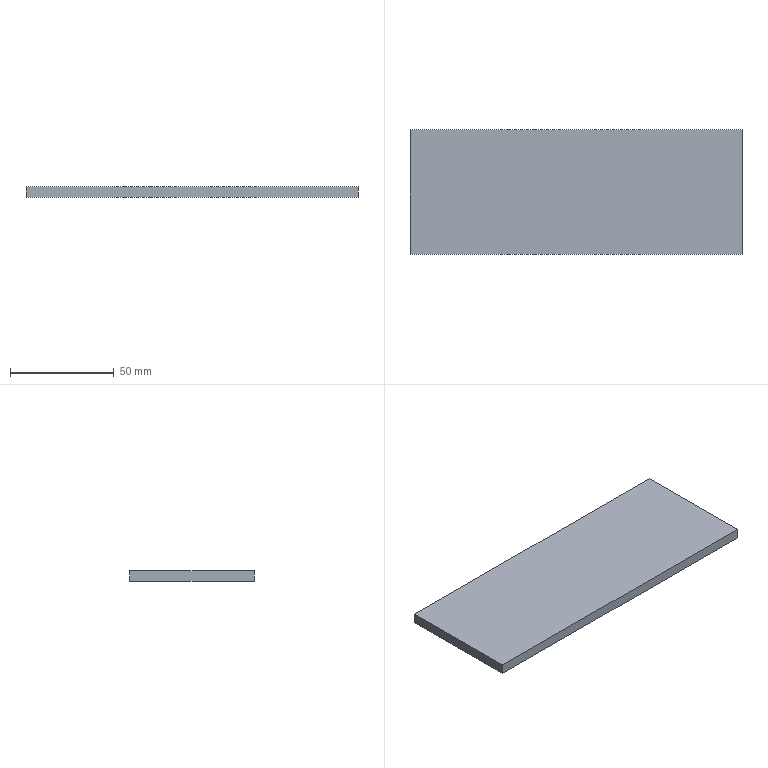Part | STEP file | Handling mechanism base plate | 1 solid | 6 faces | box 160 x 60 x 5 mm | volume 48000 mm3 | plane 6
STEP:
#1=CARTESIAN_POINT('',(80.,-30.,0.));
#2=VERTEX_POINT('',#1);
#3=CARTESIAN_POINT('',(80.,30.,0.));
#4=VERTEX_POINT('',#3);
#5=CARTESIAN_POINT('',(80.,-30.,0.));
#6=DIRECTION('',(0.,1.,0.));
#7=VECTOR('',#6,1000.);
#8=LINE('',#5,#7);
#9=EDGE_CURVE('',#2,#4,#8,.T.);
#10=ORIENTED_EDGE('',*,*,#9,.T.);
#11=CARTESIAN_POINT('',(80.,30.,5.));
#12=VERTEX_POINT('',#11);
#13=CARTESIAN_POINT('',(80.,30.,5.));
#14=DIRECTION('',(0.,0.,-1.));
#15=VECTOR('',#14,1000.);
#16=LINE('',#13,#15);
#17=EDGE_CURVE('',#12,#4,#16,.T.);
#18=ORIENTED_EDGE('',*,*,#17,.F.);
#19=CARTESIAN_POINT('',(80.,-30.,5.));
#20=VERTEX_POINT('',#19);
#21=CARTESIAN_POINT('',(80.,-30.,5.));
#22=DIRECTION('',(0.,1.,0.));
#23=VECTOR('',#22,1000.);
#24=LINE('',#21,#23);
#25=EDGE_CURVE('',#20,#12,#24,.T.);
#26=ORIENTED_EDGE('',*,*,#25,.F.);
#27=CARTESIAN_POINT('',(80.,-30.,5.));
#28=DIRECTION('',(0.,0.,-1.));
#29=VECTOR('',#28,1000.);
#30=LINE('',#27,#29);
#31=EDGE_CURVE('',#20,#2,#30,.T.);
#32=ORIENTED_EDGE('',*,*,#31,.T.);
#33=EDGE_LOOP('',(#10,#18,#26,#32));
#34=FACE_OUTER_BOUND('',#33,.T.);
#35=CARTESIAN_POINT('',(80.,-30.,5.));
#36=DIRECTION('',(-1.,0.,0.));
#37=DIRECTION('',(0.,0.,1.));
#38=AXIS2_PLACEMENT_3D('',#35,#36,#37);
#39=PLANE('',#38);
#40=ADVANCED_FACE('',(#34),#39,.F.);
#41=CARTESIAN_POINT('',(-80.,30.,0.));
#42=VERTEX_POINT('',#41);
#43=CARTESIAN_POINT('',(-80.,30.,0.));
#44=DIRECTION('',(-1.,0.,0.));
#45=VECTOR('',#44,1000.);
#46=LINE('',#43,#45);
#47=EDGE_CURVE('',#4,#42,#46,.T.);
#48=ORIENTED_EDGE('',*,*,#47,.T.);
#49=CARTESIAN_POINT('',(-80.,30.,5.));
#50=VERTEX_POINT('',#49);
#51=CARTESIAN_POINT('',(-80.,30.,5.));
#52=DIRECTION('',(0.,0.,-1.));
#53=VECTOR('',#52,1000.);
#54=LINE('',#51,#53);
#55=EDGE_CURVE('',#50,#42,#54,.T.);
#56=ORIENTED_EDGE('',*,*,#55,.F.);
#57=CARTESIAN_POINT('',(-80.,30.,5.));
#58=DIRECTION('',(-1.,0.,0.));
#59=VECTOR('',#58,1000.);
#60=LINE('',#57,#59);
#61=EDGE_CURVE('',#12,#50,#60,.T.);
#62=ORIENTED_EDGE('',*,*,#61,.F.);
#63=ORIENTED_EDGE('',*,*,#17,.T.);
#64=EDGE_LOOP('',(#48,#56,#62,#63));
#65=FACE_OUTER_BOUND('',#64,.T.);
#66=CARTESIAN_POINT('',(-80.,30.,5.));
#67=DIRECTION('',(0.,-1.,0.));
#68=DIRECTION('',(0.,0.,-1.));
#69=AXIS2_PLACEMENT_3D('',#66,#67,#68);
#70=PLANE('',#69);
#71=ADVANCED_FACE('',(#65),#70,.F.);
#72=CARTESIAN_POINT('',(-80.,-30.,0.));
#73=VERTEX_POINT('',#72);
#74=CARTESIAN_POINT('',(-80.,-30.,0.));
#75=DIRECTION('',(0.,-1.,0.));
#76=VECTOR('',#75,1000.);
#77=LINE('',#74,#76);
#78=EDGE_CURVE('',#42,#73,#77,.T.);
#79=ORIENTED_EDGE('',*,*,#78,.T.);
#80=CARTESIAN_POINT('',(-80.,-30.,5.));
#81=VERTEX_POINT('',#80);
#82=CARTESIAN_POINT('',(-80.,-30.,5.));
#83=DIRECTION('',(0.,0.,-1.));
#84=VECTOR('',#83,1000.);
#85=LINE('',#82,#84);
#86=EDGE_CURVE('',#81,#73,#85,.T.);
#87=ORIENTED_EDGE('',*,*,#86,.F.);
#88=CARTESIAN_POINT('',(-80.,-30.,5.));
#89=DIRECTION('',(0.,-1.,0.));
#90=VECTOR('',#89,1000.);
#91=LINE('',#88,#90);
#92=EDGE_CURVE('',#50,#81,#91,.T.);
#93=ORIENTED_EDGE('',*,*,#92,.F.);
#94=ORIENTED_EDGE('',*,*,#55,.T.);
#95=EDGE_LOOP('',(#79,#87,#93,#94));
#96=FACE_OUTER_BOUND('',#95,.T.);
#97=CARTESIAN_POINT('',(-80.,-30.,5.));
#98=DIRECTION('',(1.,0.,0.));
#99=DIRECTION('',(0.,0.,-1.));
#100=AXIS2_PLACEMENT_3D('',#97,#98,#99);
#101=PLANE('',#100);
#102=ADVANCED_FACE('',(#96),#101,.F.);
#103=CARTESIAN_POINT('',(-80.,-30.,0.));
#104=DIRECTION('',(1.,0.,0.));
#105=VECTOR('',#104,1000.);
#106=LINE('',#103,#105);
#107=EDGE_CURVE('',#73,#2,#106,.T.);
#108=ORIENTED_EDGE('',*,*,#107,.T.);
#109=ORIENTED_EDGE('',*,*,#31,.F.);
#110=CARTESIAN_POINT('',(-80.,-30.,5.));
#111=DIRECTION('',(1.,0.,0.));
#112=VECTOR('',#111,1000.);
#113=LINE('',#110,#112);
#114=EDGE_CURVE('',#81,#20,#113,.T.);
#115=ORIENTED_EDGE('',*,*,#114,.F.);
#116=ORIENTED_EDGE('',*,*,#86,.T.);
#117=EDGE_LOOP('',(#108,#109,#115,#116));
#118=FACE_OUTER_BOUND('',#117,.T.);
#119=CARTESIAN_POINT('',(-80.,-30.,5.));
#120=DIRECTION('',(0.,1.,0.));
#121=DIRECTION('',(0.,0.,1.));
#122=AXIS2_PLACEMENT_3D('',#119,#120,#121);
#123=PLANE('',#122);
#124=ADVANCED_FACE('',(#118),#123,.F.);
#125=ORIENTED_EDGE('',*,*,#25,.T.);
#126=ORIENTED_EDGE('',*,*,#61,.T.);
#127=ORIENTED_EDGE('',*,*,#92,.T.);
#128=ORIENTED_EDGE('',*,*,#114,.T.);
#129=EDGE_LOOP('',(#125,#126,#127,#128));
#130=FACE_OUTER_BOUND('',#129,.T.);
#131=CARTESIAN_POINT('',(0.,0.,5.));
#132=DIRECTION('',(0.,0.,-1.));
#133=DIRECTION('',(-1.,0.,0.));
#134=AXIS2_PLACEMENT_3D('',#131,#132,#133);
#135=PLANE('',#134);
#136=ADVANCED_FACE('',(#130),#135,.F.);
#137=ORIENTED_EDGE('',*,*,#9,.F.);
#138=ORIENTED_EDGE('',*,*,#107,.F.);
#139=ORIENTED_EDGE('',*,*,#78,.F.);
#140=ORIENTED_EDGE('',*,*,#47,.F.);
#141=EDGE_LOOP('',(#137,#138,#139,#140));
#142=FACE_OUTER_BOUND('',#141,.T.);
#143=CARTESIAN_POINT('',(0.,0.,0.));
#144=DIRECTION('',(0.,0.,-1.));
#145=DIRECTION('',(-1.,0.,0.));
#146=AXIS2_PLACEMENT_3D('',#143,#144,#145);
#147=PLANE('',#146);
#148=ADVANCED_FACE('',(#142),#147,.T.);
#149=CLOSED_SHELL('',(#40,#71,#102,#124,#136,#148));
#150=MANIFOLD_SOLID_BREP('',#149);
#151=CARTESIAN_POINT('',(0.,0.,0.));
#152=DIRECTION('',(0.,0.,1.));
#153=DIRECTION('',(1.,0.,0.));
#154=AXIS2_PLACEMENT_3D('',#151,#152,#153);
#155=(LENGTH_UNIT()NAMED_UNIT(*)SI_UNIT(.MILLI.,.METRE.));
#156=UNCERTAINTY_MEASURE_WITH_UNIT(LENGTH_MEASURE(0.00001),#155,'','');
#157=(NAMED_UNIT(*)PLANE_ANGLE_UNIT()SI_UNIT($,.RADIAN.));
#158=(NAMED_UNIT(*)SI_UNIT($,.STERADIAN.)SOLID_ANGLE_UNIT());
#159=(GEOMETRIC_REPRESENTATION_CONTEXT(3)GLOBAL_UNCERTAINTY_ASSIGNED_CONTEXT((#156))GLOBAL_UNIT_ASSIGNED_CONTEXT((#155,#157,#158))REPRESENTATION_CONTEXT('',''));
#160=ADVANCED_BREP_SHAPE_REPRESENTATION('',(#150,#154),#159);